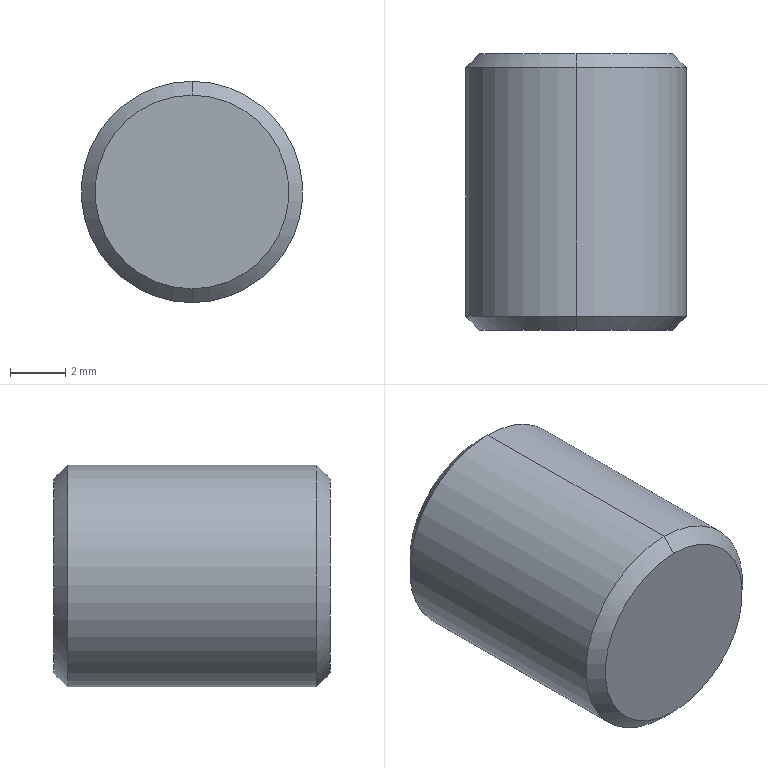Part | SolidWorks | features Chamfer 1, Extrusion 1 | 1 solid | 8 faces | box 8 x 10 x 8 mm | volume 496.633 mm3 | cone 4 | cylinder 2 | plane 2 | commonest cylinder face diameters 8 x2
STEP:
#1=CARTESIAN_POINT('',(0.,10.,3.5));
#2=VERTEX_POINT('',#1);
#3=CARTESIAN_POINT('',(0.,10.,-3.5));
#4=VERTEX_POINT('',#3);
#5=CARTESIAN_POINT('',(0.,10.,0.));
#6=DIRECTION('',(0.,1.,0.));
#7=DIRECTION('',(0.,0.,1.));
#8=AXIS2_PLACEMENT_3D('',#5,#6,#7);
#9=CIRCLE('',#8,3.5);
#10=EDGE_CURVE('',#2,#4,#9,.T.);
#11=ORIENTED_EDGE('',*,*,#10,.F.);
#12=CARTESIAN_POINT('',(0.,9.5,4.));
#13=VERTEX_POINT('',#12);
#14=CARTESIAN_POINT('',(0.,10.,3.5));
#15=DIRECTION('',(0.,-0.7071,0.7071));
#16=VECTOR('',#15,1000.);
#17=LINE('',#14,#16);
#18=EDGE_CURVE('',#2,#13,#17,.T.);
#19=ORIENTED_EDGE('',*,*,#18,.T.);
#20=CARTESIAN_POINT('',(0.,9.5,-4.));
#21=VERTEX_POINT('',#20);
#22=CARTESIAN_POINT('',(0.,9.5,0.));
#23=DIRECTION('',(0.,-1.,0.));
#24=DIRECTION('',(0.,0.,1.));
#25=AXIS2_PLACEMENT_3D('',#22,#23,#24);
#26=CIRCLE('',#25,4.);
#27=EDGE_CURVE('',#21,#13,#26,.T.);
#28=ORIENTED_EDGE('',*,*,#27,.F.);
#29=CARTESIAN_POINT('',(0.,10.,-3.5));
#30=DIRECTION('',(0.,-0.7071,-0.7071));
#31=VECTOR('',#30,1000.);
#32=LINE('',#29,#31);
#33=EDGE_CURVE('',#4,#21,#32,.T.);
#34=ORIENTED_EDGE('',*,*,#33,.F.);
#35=EDGE_LOOP('',(#11,#19,#28,#34));
#36=FACE_OUTER_BOUND('',#35,.T.);
#37=CARTESIAN_POINT('',(0.,10.,0.));
#38=DIRECTION('',(0.,-1.,0.));
#39=DIRECTION('',(0.,0.,-1.));
#40=AXIS2_PLACEMENT_3D('',#37,#38,#39);
#41=CONICAL_SURFACE('',#40,3.5,0.7854);
#42=ADVANCED_FACE('',(#36),#41,.T.);
#43=CARTESIAN_POINT('',(0.,0.,-3.5));
#44=VERTEX_POINT('',#43);
#45=CARTESIAN_POINT('',(0.,0.,3.5));
#46=VERTEX_POINT('',#45);
#47=CARTESIAN_POINT('',(0.,0.,0.));
#48=DIRECTION('',(0.,-1.,0.));
#49=DIRECTION('',(0.,0.,1.));
#50=AXIS2_PLACEMENT_3D('',#47,#48,#49);
#51=CIRCLE('',#50,3.5);
#52=EDGE_CURVE('',#44,#46,#51,.T.);
#53=ORIENTED_EDGE('',*,*,#52,.F.);
#54=CARTESIAN_POINT('',(0.,0.5,-4.));
#55=VERTEX_POINT('',#54);
#56=CARTESIAN_POINT('',(0.,0.5,-4.));
#57=DIRECTION('',(0.,0.7071,-0.7071));
#58=VECTOR('',#57,1000.);
#59=LINE('',#56,#58);
#60=EDGE_CURVE('',#44,#55,#59,.T.);
#61=ORIENTED_EDGE('',*,*,#60,.T.);
#62=CARTESIAN_POINT('',(0.,0.5,4.));
#63=VERTEX_POINT('',#62);
#64=CARTESIAN_POINT('',(0.,0.5,0.));
#65=DIRECTION('',(0.,1.,0.));
#66=DIRECTION('',(0.,0.,1.));
#67=AXIS2_PLACEMENT_3D('',#64,#65,#66);
#68=CIRCLE('',#67,4.);
#69=EDGE_CURVE('',#63,#55,#68,.T.);
#70=ORIENTED_EDGE('',*,*,#69,.F.);
#71=CARTESIAN_POINT('',(0.,0.5,4.));
#72=DIRECTION('',(0.,0.7071,0.7071));
#73=VECTOR('',#72,1000.);
#74=LINE('',#71,#73);
#75=EDGE_CURVE('',#46,#63,#74,.T.);
#76=ORIENTED_EDGE('',*,*,#75,.F.);
#77=EDGE_LOOP('',(#53,#61,#70,#76));
#78=FACE_OUTER_BOUND('',#77,.T.);
#79=CARTESIAN_POINT('',(0.,0.5,0.));
#80=DIRECTION('',(0.,1.,0.));
#81=DIRECTION('',(0.,0.,1.));
#82=AXIS2_PLACEMENT_3D('',#79,#80,#81);
#83=CONICAL_SURFACE('',#82,4.,0.7854);
#84=ADVANCED_FACE('',(#78),#83,.T.);
#85=ORIENTED_EDGE('',*,*,#27,.T.);
#86=CARTESIAN_POINT('',(0.,10.,4.));
#87=DIRECTION('',(0.,-1.,0.));
#88=VECTOR('',#87,1000.);
#89=LINE('',#86,#88);
#90=EDGE_CURVE('',#13,#63,#89,.T.);
#91=ORIENTED_EDGE('',*,*,#90,.T.);
#92=ORIENTED_EDGE('',*,*,#69,.T.);
#93=CARTESIAN_POINT('',(0.,10.,-4.));
#94=DIRECTION('',(0.,-1.,0.));
#95=VECTOR('',#94,1000.);
#96=LINE('',#93,#95);
#97=EDGE_CURVE('',#21,#55,#96,.T.);
#98=ORIENTED_EDGE('',*,*,#97,.F.);
#99=EDGE_LOOP('',(#85,#91,#92,#98));
#100=FACE_OUTER_BOUND('',#99,.T.);
#101=CARTESIAN_POINT('',(0.,10.,0.));
#102=DIRECTION('',(0.,-1.,0.));
#103=DIRECTION('',(0.,0.,-1.));
#104=AXIS2_PLACEMENT_3D('',#101,#102,#103);
#105=CYLINDRICAL_SURFACE('',#104,4.);
#106=ADVANCED_FACE('',(#100),#105,.T.);
#107=ORIENTED_EDGE('',*,*,#90,.F.);
#108=CARTESIAN_POINT('',(0.,9.5,0.));
#109=DIRECTION('',(0.,-1.,0.));
#110=DIRECTION('',(0.,0.,1.));
#111=AXIS2_PLACEMENT_3D('',#108,#109,#110);
#112=CIRCLE('',#111,4.);
#113=EDGE_CURVE('',#13,#21,#112,.T.);
#114=ORIENTED_EDGE('',*,*,#113,.T.);
#115=ORIENTED_EDGE('',*,*,#97,.T.);
#116=CARTESIAN_POINT('',(0.,0.5,0.));
#117=DIRECTION('',(0.,1.,0.));
#118=DIRECTION('',(0.,0.,1.));
#119=AXIS2_PLACEMENT_3D('',#116,#117,#118);
#120=CIRCLE('',#119,4.);
#121=EDGE_CURVE('',#55,#63,#120,.T.);
#122=ORIENTED_EDGE('',*,*,#121,.T.);
#123=EDGE_LOOP('',(#107,#114,#115,#122));
#124=FACE_OUTER_BOUND('',#123,.T.);
#125=CARTESIAN_POINT('',(0.,10.,0.));
#126=DIRECTION('',(0.,-1.,0.));
#127=DIRECTION('',(0.,0.,-1.));
#128=AXIS2_PLACEMENT_3D('',#125,#126,#127);
#129=CYLINDRICAL_SURFACE('',#128,4.);
#130=ADVANCED_FACE('',(#124),#129,.T.);
#131=CARTESIAN_POINT('',(0.,10.,0.));
#132=DIRECTION('',(0.,1.,0.));
#133=DIRECTION('',(0.,0.,1.));
#134=AXIS2_PLACEMENT_3D('',#131,#132,#133);
#135=CIRCLE('',#134,3.5);
#136=EDGE_CURVE('',#4,#2,#135,.T.);
#137=ORIENTED_EDGE('',*,*,#136,.T.);
#138=ORIENTED_EDGE('',*,*,#10,.T.);
#139=EDGE_LOOP('',(#137,#138));
#140=FACE_OUTER_BOUND('',#139,.T.);
#141=CARTESIAN_POINT('',(0.,10.,0.));
#142=DIRECTION('',(0.,1.,0.));
#143=DIRECTION('',(0.,0.,1.));
#144=AXIS2_PLACEMENT_3D('',#141,#142,#143);
#145=PLANE('',#144);
#146=ADVANCED_FACE('',(#140),#145,.T.);
#147=CARTESIAN_POINT('',(0.,0.,0.));
#148=DIRECTION('',(0.,-1.,0.));
#149=DIRECTION('',(0.,0.,1.));
#150=AXIS2_PLACEMENT_3D('',#147,#148,#149);
#151=CIRCLE('',#150,3.5);
#152=EDGE_CURVE('',#46,#44,#151,.T.);
#153=ORIENTED_EDGE('',*,*,#152,.T.);
#154=ORIENTED_EDGE('',*,*,#52,.T.);
#155=EDGE_LOOP('',(#153,#154));
#156=FACE_OUTER_BOUND('',#155,.T.);
#157=CARTESIAN_POINT('',(0.,0.,0.));
#158=DIRECTION('',(0.,1.,0.));
#159=DIRECTION('',(0.,0.,1.));
#160=AXIS2_PLACEMENT_3D('',#157,#158,#159);
#161=PLANE('',#160);
#162=ADVANCED_FACE('',(#156),#161,.F.);
#163=ORIENTED_EDGE('',*,*,#60,.F.);
#164=ORIENTED_EDGE('',*,*,#152,.F.);
#165=ORIENTED_EDGE('',*,*,#75,.T.);
#166=ORIENTED_EDGE('',*,*,#121,.F.);
#167=EDGE_LOOP('',(#163,#164,#165,#166));
#168=FACE_OUTER_BOUND('',#167,.T.);
#169=CARTESIAN_POINT('',(0.,0.5,0.));
#170=DIRECTION('',(0.,1.,0.));
#171=DIRECTION('',(0.,0.,1.));
#172=AXIS2_PLACEMENT_3D('',#169,#170,#171);
#173=CONICAL_SURFACE('',#172,4.,0.7854);
#174=ADVANCED_FACE('',(#168),#173,.T.);
#175=ORIENTED_EDGE('',*,*,#18,.F.);
#176=ORIENTED_EDGE('',*,*,#136,.F.);
#177=ORIENTED_EDGE('',*,*,#33,.T.);
#178=ORIENTED_EDGE('',*,*,#113,.F.);
#179=EDGE_LOOP('',(#175,#176,#177,#178));
#180=FACE_OUTER_BOUND('',#179,.T.);
#181=CARTESIAN_POINT('',(0.,10.,0.));
#182=DIRECTION('',(0.,-1.,0.));
#183=DIRECTION('',(0.,0.,-1.));
#184=AXIS2_PLACEMENT_3D('',#181,#182,#183);
#185=CONICAL_SURFACE('',#184,3.5,0.7854);
#186=ADVANCED_FACE('',(#180),#185,.T.);
#187=CLOSED_SHELL('',(#42,#84,#106,#130,#146,#162,#174,#186));
#188=MANIFOLD_SOLID_BREP('',#187);
#189=CARTESIAN_POINT('',(0.,0.,0.));
#190=DIRECTION('',(0.,0.,1.));
#191=DIRECTION('',(1.,0.,0.));
#192=AXIS2_PLACEMENT_3D('',#189,#190,#191);
#193=(LENGTH_UNIT()NAMED_UNIT(*)SI_UNIT(.MILLI.,.METRE.));
#194=UNCERTAINTY_MEASURE_WITH_UNIT(LENGTH_MEASURE(0.00001),#193,'','');
#195=(NAMED_UNIT(*)PLANE_ANGLE_UNIT()SI_UNIT($,.RADIAN.));
#196=(NAMED_UNIT(*)SI_UNIT($,.STERADIAN.)SOLID_ANGLE_UNIT());
#197=(GEOMETRIC_REPRESENTATION_CONTEXT(3)GLOBAL_UNCERTAINTY_ASSIGNED_CONTEXT((#194))GLOBAL_UNIT_ASSIGNED_CONTEXT((#193,#195,#196))REPRESENTATION_CONTEXT('',''));
#198=ADVANCED_BREP_SHAPE_REPRESENTATION('',(#188,#192),#197);